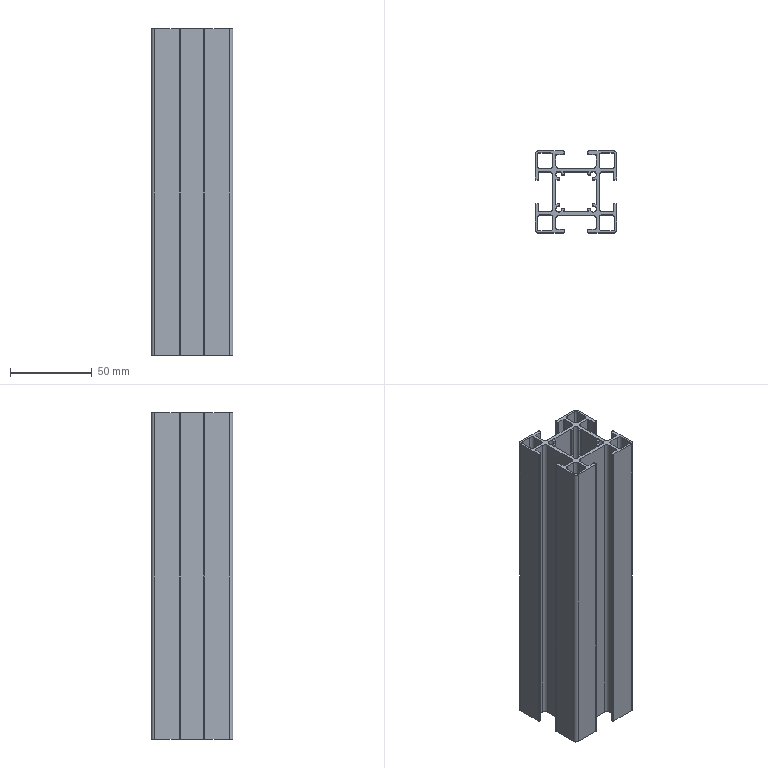Part | STEP file | 46A-00006CC11-200mm | 1 solid | 142 faces | box 50 x 50 x 200 mm | volume 117498 mm3 | cylinder 84 | plane 58 | commonest cylinder face diameters 1 x24 4 x24 1.5 x16 3.7 x8 6.7 x8 2 x4